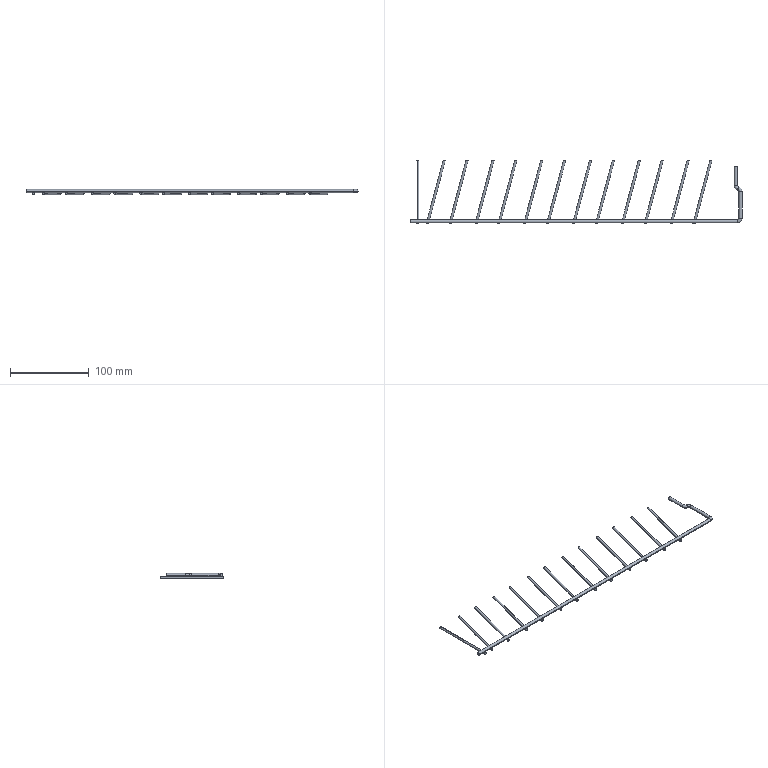Part | STEP file | ZXW722-L-178-C_14_1_1 | 1 solid | 68 faces | box 421.95 x 80.725 x 6.4 mm | volume 12477 mm3 | cylinder 34 | plane 28 | torus 6 | commonest cylinder face diameters 2.8 x26 3.9 x8